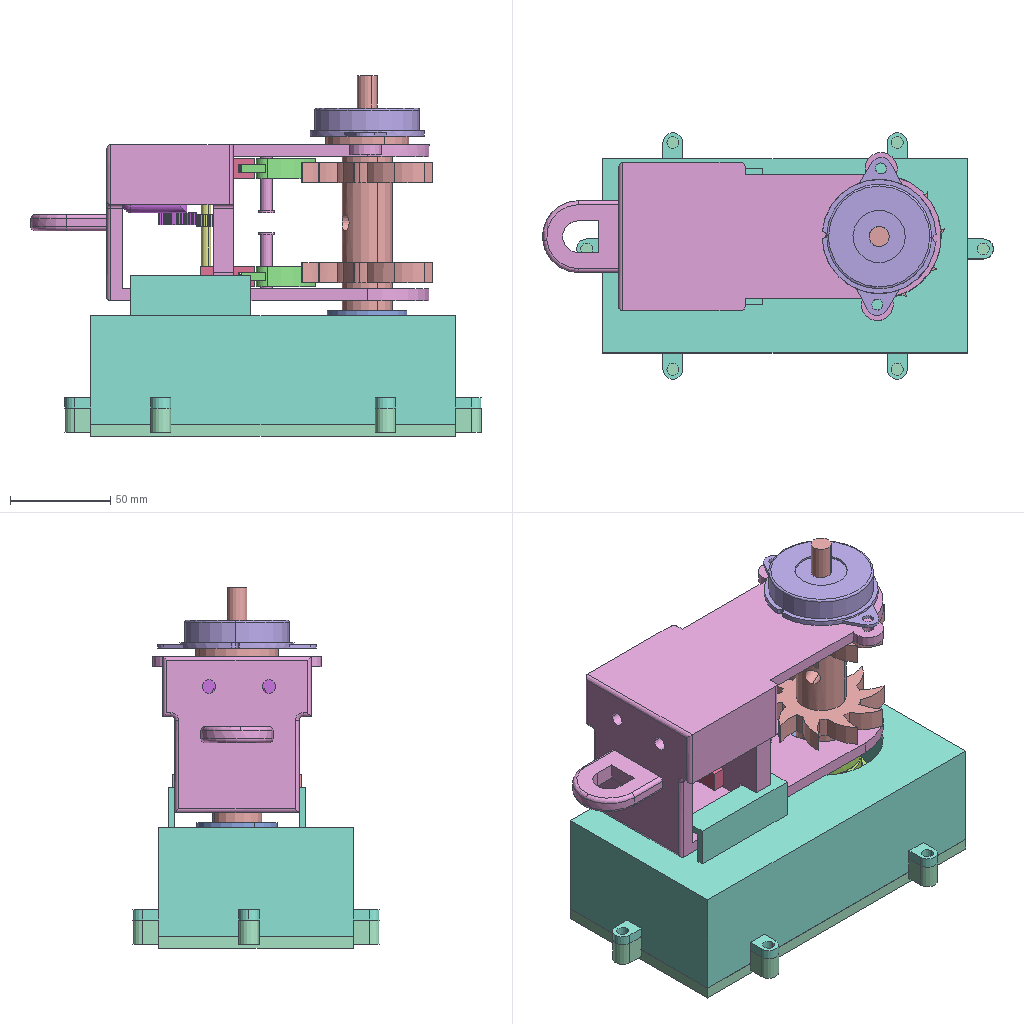Assembly | SolidWorks | 11 different items | 14 placed | box 225 x 123 x 180 mm
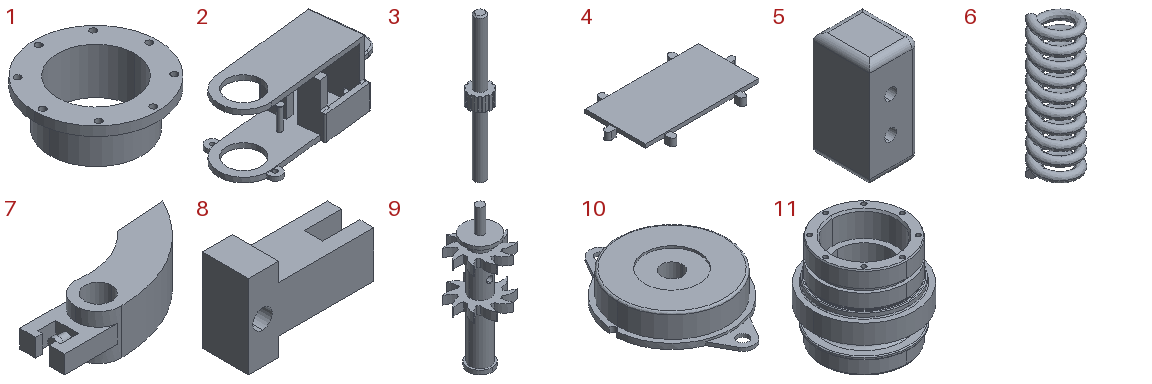Parts list (item | quantity | size | volume | features):
1 | x1 | 40 x 40 x 15 mm | 4809 mm3 | features ICE 2, Cut 1, Extrusion 1
2 | x1 | 198.087 x 92.564 x 78 mm | 194548 mm3 | features ICE 11, MirrorPattern 3, Fillet 2, Extrusion 1, HoleWzd 1, MirrorSolid 1
3 | x1 | 9.896 x 9.896 x 64 mm | 1479 mm3 | features Extrusion 1, ICE 1, MirrorPattern 1, StudWizard 1
4 | x1 | 208 x 123 x 14 mm | 114511 mm3 | features Extrusion 1, ICE 1
5 | x1 | 34 x 36.976 x 60 mm | 53977 mm3 | features Extrusion 1, Fillet 1, HoleWzd 1, ICE 1
6 | x2 | 3.2 x 3.2 x 10.596 mm | 23.105 mm3 | features Helix 1, Sweep 1
7 | x2 | 37.304 x 15.525 x 10 mm | 2448 mm3 | features ICE 6, Extrusion 1
8 | x2 | 27 x 10 x 18 mm | 2677 mm3 | features ICE 7, Extrusion 1, HoleWzd 1, MirrorPattern 1
9 | x1 | 65.926 x 62.827 x 170.5 mm | 102049 mm3 | features ICE 7, Cut 1, Extrusion 1, MirrorSolid 1
10 | x1 | 56.886 x 79 x 13.8 mm | 28746 mm3 | features BaseBody 1
11 | x1 | 47.505 x 47.505 x 45.25 mm | 32627 mm3 | features BaseBody 1
Mates (type | each side: item.copy, entity, surface, feature):
Concentric | assembly face | 9.1 face cylinder Boss-Extrude1
Coincident | assembly face | 9.1 face plane Boss-Extrude1
Concentric | 9.1 face cylinder Boss-Extrude1 | 1.1 face cylinder Boss-Extrude1
Coincident | assembly face | 1.1 face plane Boss-Extrude1
Concentric | assembly edge | 1.1 edge
Concentric | 9.1 face cylinder Boss-Extrude1 | assembly face
Concentric | 9.1 face cylinder Mirror1 | assembly face
Coincident | 9.1 face plane Mirror1 | assembly face
Coincident | 9.1 face plane Boss-Extrude4 | assembly face
InPlace | assembly face | 2.1 plane
Concentric | 9.1 face cylinder Boss-Extrude7 | 10.1 face cylinder Input1
Coincident | 9.1 face plane Boss-Extrude6 | 10.1 face plane Input1
Concentric | 2.1 face cylinder Mirror1 | 7.1 face cylinder Boss-Extrude1
Parallel | 7.1 face plane Boss-Extrude3 | 8.1 face plane Cut-Extrude1
Coincident | 2.1 face plane Mirror5 | 8.1 face plane Boss-Extrude1
Coincident | 2.1 face plane Boss-Extrude4 | 8.1 face plane Boss-Extrude3
Coincident | 7.1 face plane Boss-Extrude3 | 8.1 face plane Cut-Extrude1
Concentric | 7.1 face cylinder Boss-Extrude4 | 6.1 select_type:24
Coincident | 7.1 face plane Cut-Extrude3 | 6.1 select_type:24
LimitDistanceDim | 7.1 face plane Boss-Extrude1 | 2.1 face plane Mirror1
Parallel | 8.1 face plane Boss-Extrude1 | 8.2 face plane Boss-Extrude1
Coincident | 2.1 face plane Boss-Extrude4 | 8.2 face plane Boss-Extrude3
Coincident | 2.1 face plane Cut-Extrude3 | 8.2 face plane Boss-Extrude1
Concentric | 2.1 face cylinder Boss-Extrude3 | 7.2 face cylinder Boss-Extrude1
Concentric | 7.2 face cylinder Boss-Extrude4 | 6.2 select_type:24
Coincident | 7.2 face plane Cut-Extrude3 | 6.2 select_type:24
Coincident | 7.2 face plane Boss-Extrude3 | 8.2 face plane Cut-Extrude1
LimitDistanceDim | 7.2 face plane Boss-Extrude1 | 2.1 face plane Boss-Extrude6
Concentric | 8.2 edge | 3.1 edge
Coincident | 2.1 face plane Mirror1 | 3.1 face plane Boss-Extrude1
Parallel | 2.1 face plane Boss-Extrude1 | 5.1 face plane Boss-Extrude1
Coincident | 2.1 face plane Boss-Extrude2 | 5.1 face plane Boss-Extrude1
Coincident | 2.1 face plane Mirror1 | 5.1 face plane Boss-Extrude1
Coincident | 2.1 face plane Boss-Extrude1 | 5.1 face plane Boss-Extrude1
Concentric | 2.1 face cylinder Tap Drill for M8 Tap1 | assembly face | 2 times
Coincident | 2.1 face plane Boss-Extrude1 | assembly edge | 2 times
Concentric | 2.1 face cylinder Boss-Extrude8 | assembly face | 2 times
Coincident | 10.1 face plane Input1 | assembly edge | 2 times